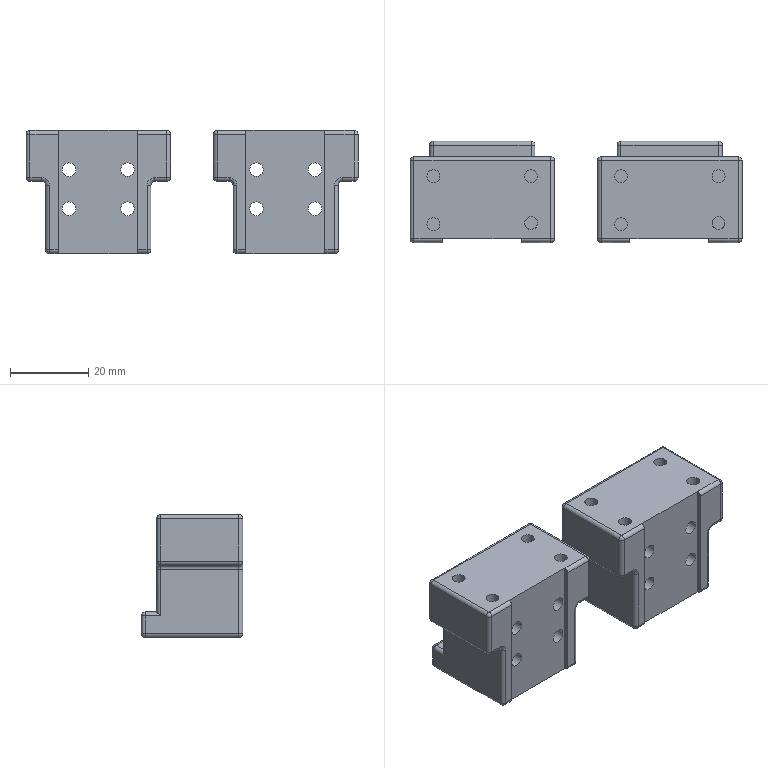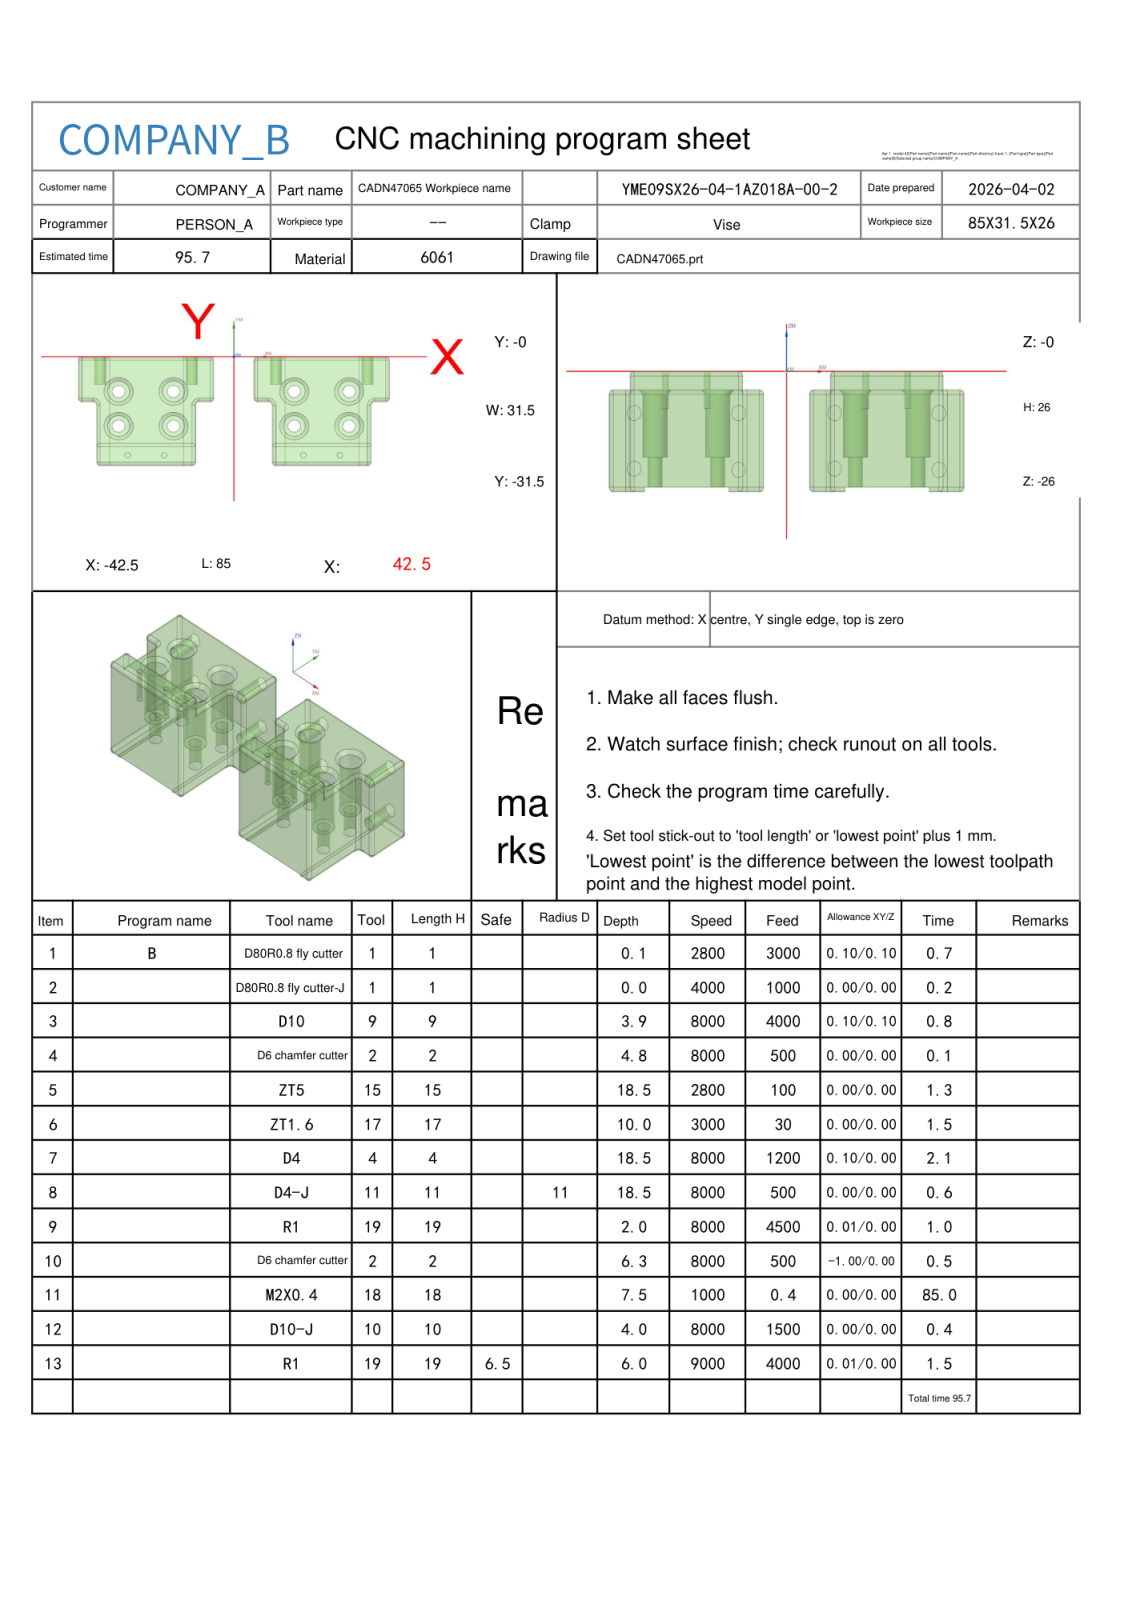NC program | NX | posted by the shop | part box 85 x 26 x 31.5 mm
Lines 10969 to 12542 of 12542:
N10 T02 M06
(D6 chamfer cutter  D=6. R=0. H=02 ce=0.00 di=0.00)
G00 G90 G54 X-29.011 Y-28.455 M03 S8000
G43 H02 Z20.
M08
G98 G81 X-29.011 Y-28.455 Z-1.2 R3. F500.
X-19.011
X18.989
X28.989
G80
G00 Z20.
G00 G90 X-33.191 Y-20.222 M03 S8000
Z20.
Z-1.5
G01 X-33.173 Y-20.379 Z-1.558 F500.
X-33.097 Y-20.648 Z-1.659
X-32.977 Y-20.902 Z-1.761
X-32.818 Y-21.132 Z-1.863
X-32.623 Y-21.333 Z-1.965
X-32.397 Y-21.499 Z-2.067
X-32.148 Y-21.626 Z-2.169
X-31.881 Y-21.71 Z-2.271
X-31.604 Y-21.75 Z-2.373
X-31.401 Z-2.447
X-31.124 Y-21.71 Z-2.548
X-30.857 Y-21.626 Z-2.65
X-30.608 Y-21.499 Z-2.752
X-30.382 Y-21.333 Z-2.854
X-30.187 Y-21.132 Z-2.956
X-30.028 Y-20.902 Z-3.058
X-29.908 Y-20.648 Z-3.16
X-29.832 Y-20.379 Z-3.262
X-29.8 Y-20.101 Z-3.364
X-29.815 Y-19.821 Z-3.466
X-29.875 Y-19.547 Z-3.568
X-29.98 Y-19.288 Z-3.67
X-30.081 Y-19.113 Z-3.743
X-30.254 Y-18.892 Z-3.845
X-30.46 Y-18.703 Z-3.947
X-30.695 Y-18.551 Z-4.049
X-30.952 Y-18.439 Z-4.151
X-31.223 Y-18.37 Z-4.253
X-31.502 Y-18.347 Z-4.355
X-31.782 Y-18.37 Z-4.457
X-32.053 Y-18.439 Z-4.559
X-32.31 Y-18.551 Z-4.661
X-32.545 Y-18.703 Z-4.763
X-32.751 Y-18.892 Z-4.865
X-32.924 Y-19.113 Z-4.967
X-33.025 Y-19.288 Z-5.04
X-33.13 Y-19.547 Z-5.142
X-33.19 Y-19.821 Z-5.244
X-33.205 Y-20.101 Z-5.346
X-33.173 Y-20.379 Z-5.448
X-33.097 Y-20.648 Z-5.55
X-32.977 Y-20.902 Z-5.652
X-32.818 Y-21.132 Z-5.754
X-32.623 Y-21.333 Z-5.856
X-32.397 Y-21.499 Z-5.957
X-32.148 Y-21.626 Z-6.059
X-31.881 Y-21.71 Z-6.161
X-31.604 Y-21.75 Z-6.263
X-31.502 Z-6.3
G03 X-29.802 Y-20.05 I0.0 J1.7
X-31.502 Y-18.35 I-1.7 J0.0
X-33.202 Y-20.05 I0.0 J-1.7
X-31.502 Y-21.75 I1.7 J0.0
X-31.01 Y-21.677 I0.0 J1.7
G01 Z-3.8
G00 Z20.
X-33.191 Y-10.222
Z-1.5
G01 X-33.173 Y-10.379 Z-1.558
X-33.097 Y-10.648 Z-1.659
X-32.977 Y-10.902 Z-1.761
X-32.818 Y-11.132 Z-1.863
X-32.623 Y-11.333 Z-1.965
X-32.397 Y-11.499 Z-2.067
X-32.148 Y-11.626 Z-2.169
X-31.881 Y-11.71 Z-2.271
X-31.604 Y-11.75 Z-2.373
X-31.401 Z-2.447
X-31.124 Y-11.71 Z-2.548
X-30.857 Y-11.626 Z-2.65
X-30.608 Y-11.499 Z-2.752
X-30.382 Y-11.333 Z-2.854
X-30.187 Y-11.132 Z-2.956
X-30.028 Y-10.902 Z-3.058
X-29.908 Y-10.648 Z-3.16
X-29.832 Y-10.379 Z-3.262
X-29.8 Y-10.101 Z-3.364
X-29.815 Y-9.821 Z-3.466
X-29.875 Y-9.547 Z-3.568
X-29.98 Y-9.288 Z-3.67
X-30.081 Y-9.113 Z-3.743
X-30.254 Y-8.892 Z-3.845
X-30.46 Y-8.703 Z-3.947
X-30.695 Y-8.551 Z-4.049
X-30.952 Y-8.439 Z-4.151
X-31.223 Y-8.37 Z-4.253
X-31.502 Y-8.347 Z-4.355
X-31.782 Y-8.37 Z-4.457
X-32.053 Y-8.439 Z-4.559
X-32.31 Y-8.551 Z-4.661
X-32.545 Y-8.703 Z-4.763
X-32.751 Y-8.892 Z-4.865
X-32.924 Y-9.113 Z-4.967
X-33.025 Y-9.288 Z-5.04
X-33.13 Y-9.547 Z-5.142
X-33.19 Y-9.821 Z-5.244
X-33.205 Y-10.101 Z-5.346
X-33.173 Y-10.379 Z-5.448
X-33.097 Y-10.648 Z-5.55
X-32.977 Y-10.902 Z-5.652
X-32.818 Y-11.132 Z-5.754
X-32.623 Y-11.333 Z-5.856
X-32.397 Y-11.499 Z-5.957
X-32.148 Y-11.626 Z-6.059
X-31.881 Y-11.71 Z-6.161
X-31.604 Y-11.75 Z-6.263
X-31.502 Z-6.3
G03 X-29.802 Y-10.05 I0.0 J1.7
X-31.502 Y-8.35 I-1.7 J0.0
X-33.202 Y-10.05 I0.0 J-1.7
X-31.502 Y-11.75 I1.7 J0.0
X-31.01 Y-11.677 I0.0 J1.7
G01 Z-3.8
G00 Z20.
X-18.191 Y-10.222
Z-1.5
G01 X-18.173 Y-10.379 Z-1.558
X-18.097 Y-10.648 Z-1.659
X-17.977 Y-10.902 Z-1.761
X-17.818 Y-11.132 Z-1.863
X-17.623 Y-11.333 Z-1.965
X-17.397 Y-11.499 Z-2.067
X-17.148 Y-11.626 Z-2.169
X-16.881 Y-11.71 Z-2.271
X-16.604 Y-11.75 Z-2.373
X-16.401 Z-2.447
X-16.124 Y-11.71 Z-2.548
X-15.857 Y-11.626 Z-2.65
X-15.608 Y-11.499 Z-2.752
X-15.382 Y-11.333 Z-2.854
X-15.187 Y-11.132 Z-2.956
X-15.028 Y-10.902 Z-3.058
X-14.908 Y-10.648 Z-3.16
X-14.832 Y-10.379 Z-3.262
X-14.8 Y-10.101 Z-3.364
X-14.815 Y-9.821 Z-3.466
X-14.875 Y-9.547 Z-3.568
X-14.98 Y-9.288 Z-3.67
X-15.081 Y-9.113 Z-3.743
X-15.254 Y-8.892 Z-3.845
X-15.46 Y-8.703 Z-3.947
X-15.695 Y-8.551 Z-4.049
X-15.952 Y-8.439 Z-4.151
X-16.223 Y-8.37 Z-4.253
X-16.502 Y-8.347 Z-4.355
X-16.782 Y-8.37 Z-4.457
X-17.053 Y-8.439 Z-4.559
X-17.31 Y-8.551 Z-4.661
X-17.545 Y-8.703 Z-4.763
X-17.751 Y-8.892 Z-4.865
X-17.924 Y-9.113 Z-4.967
X-18.025 Y-9.288 Z-5.04
X-18.13 Y-9.547 Z-5.142
X-18.19 Y-9.821 Z-5.244
X-18.205 Y-10.101 Z-5.346
X-18.173 Y-10.379 Z-5.448
X-18.097 Y-10.648 Z-5.55
X-17.977 Y-10.902 Z-5.652
X-17.818 Y-11.132 Z-5.754
X-17.623 Y-11.333 Z-5.856
X-17.397 Y-11.499 Z-5.957
X-17.148 Y-11.626 Z-6.059
X-16.881 Y-11.71 Z-6.161
X-16.604 Y-11.75 Z-6.263
X-16.502 Z-6.3
G03 X-14.802 Y-10.05 I0.0 J1.7
X-16.502 Y-8.35 I-1.7 J0.0
X-18.202 Y-10.05 I0.0 J-1.7
X-16.502 Y-11.75 I1.7 J0.0
X-16.01 Y-11.677 I0.0 J1.7
G01 Z-3.8
G00 Z20.
X-18.191 Y-20.222
Z-1.5
G01 X-18.173 Y-20.379 Z-1.558
X-18.097 Y-20.648 Z-1.659
X-17.977 Y-20.902 Z-1.761
X-17.818 Y-21.132 Z-1.863
X-17.623 Y-21.333 Z-1.965
X-17.397 Y-21.499 Z-2.067
X-17.148 Y-21.626 Z-2.169
X-16.881 Y-21.71 Z-2.271
X-16.604 Y-21.75 Z-2.373
X-16.401 Z-2.447
X-16.124 Y-21.71 Z-2.548
X-15.857 Y-21.626 Z-2.65
X-15.608 Y-21.499 Z-2.752
X-15.382 Y-21.333 Z-2.854
X-15.187 Y-21.132 Z-2.956
X-15.028 Y-20.902 Z-3.058
X-14.908 Y-20.648 Z-3.16
X-14.832 Y-20.379 Z-3.262
X-14.8 Y-20.101 Z-3.364
X-14.815 Y-19.821 Z-3.466
X-14.875 Y-19.547 Z-3.568
X-14.98 Y-19.288 Z-3.67
X-15.081 Y-19.113 Z-3.743
X-15.254 Y-18.892 Z-3.845
X-15.46 Y-18.703 Z-3.947
X-15.695 Y-18.551 Z-4.049
X-15.952 Y-18.439 Z-4.151
X-16.223 Y-18.37 Z-4.253
X-16.502 Y-18.347 Z-4.355
X-16.782 Y-18.37 Z-4.457
X-17.053 Y-18.439 Z-4.559
X-17.31 Y-18.551 Z-4.661
X-17.545 Y-18.703 Z-4.763
X-17.751 Y-18.892 Z-4.865
X-17.924 Y-19.113 Z-4.967
X-18.025 Y-19.288 Z-5.04
X-18.13 Y-19.547 Z-5.142
X-18.19 Y-19.821 Z-5.244
X-18.205 Y-20.101 Z-5.346
X-18.173 Y-20.379 Z-5.448
X-18.097 Y-20.648 Z-5.55
X-17.977 Y-20.902 Z-5.652
X-17.818 Y-21.132 Z-5.754
X-17.623 Y-21.333 Z-5.856
X-17.397 Y-21.499 Z-5.957
X-17.148 Y-21.626 Z-6.059
X-16.881 Y-21.71 Z-6.161
X-16.604 Y-21.75 Z-6.263
X-16.502 Z-6.3
G03 X-14.802 Y-20.05 I0.0 J1.7
X-16.502 Y-18.35 I-1.7 J0.0
X-18.202 Y-20.05 I0.0 J-1.7
X-16.502 Y-21.75 I1.7 J0.0
X-16.01 Y-21.677 I0.0 J1.7
G01 Z-3.8
G00 Z20.
X14.809 Y-20.222
Z-1.5
G01 X14.827 Y-20.379 Z-1.558
X14.903 Y-20.648 Z-1.659
X15.023 Y-20.902 Z-1.761
X15.182 Y-21.132 Z-1.863
X15.377 Y-21.333 Z-1.965
X15.603 Y-21.499 Z-2.067
X15.852 Y-21.626 Z-2.169
X16.119 Y-21.71 Z-2.271
X16.396 Y-21.75 Z-2.373
X16.599 Z-2.447
X16.876 Y-21.71 Z-2.548
X17.143 Y-21.626 Z-2.65
X17.392 Y-21.499 Z-2.752
X17.618 Y-21.333 Z-2.854
X17.813 Y-21.132 Z-2.956
X17.972 Y-20.902 Z-3.058
X18.092 Y-20.648 Z-3.16
X18.168 Y-20.379 Z-3.262
X18.2 Y-20.101 Z-3.364
X18.185 Y-19.821 Z-3.466
X18.125 Y-19.547 Z-3.568
X18.02 Y-19.288 Z-3.67
X17.919 Y-19.113 Z-3.743
X17.746 Y-18.892 Z-3.845
X17.54 Y-18.703 Z-3.947
X17.305 Y-18.551 Z-4.049
X17.048 Y-18.439 Z-4.151
X16.777 Y-18.37 Z-4.253
X16.498 Y-18.347 Z-4.355
X16.218 Y-18.37 Z-4.457
X15.947 Y-18.439 Z-4.559
X15.69 Y-18.551 Z-4.661
X15.455 Y-18.703 Z-4.763
X15.249 Y-18.892 Z-4.865
X15.076 Y-19.113 Z-4.967
X14.975 Y-19.288 Z-5.04
X14.87 Y-19.547 Z-5.142
X14.81 Y-19.821 Z-5.244
X14.795 Y-20.101 Z-5.346
X14.827 Y-20.379 Z-5.448
X14.903 Y-20.648 Z-5.55
X15.023 Y-20.902 Z-5.652
X15.182 Y-21.132 Z-5.754
X15.377 Y-21.333 Z-5.856
X15.603 Y-21.499 Z-5.957
X15.852 Y-21.626 Z-6.059
X16.119 Y-21.71 Z-6.161
X16.396 Y-21.75 Z-6.263
X16.498 Z-6.3
G03 X18.198 Y-20.05 I0.0 J1.7
X16.498 Y-18.35 I-1.7 J0.0
X14.798 Y-20.05 I0.0 J-1.7
X16.498 Y-21.75 I1.7 J0.0
X16.99 Y-21.677 I0.0 J1.7
G01 Z-3.8
G00 Z20.
X14.809 Y-10.222
Z-1.5
G01 X14.827 Y-10.379 Z-1.558
X14.903 Y-10.648 Z-1.659
X15.023 Y-10.902 Z-1.761
X15.182 Y-11.132 Z-1.863
X15.377 Y-11.333 Z-1.965
X15.603 Y-11.499 Z-2.067
X15.852 Y-11.626 Z-2.169
X16.119 Y-11.71 Z-2.271
X16.396 Y-11.75 Z-2.373
X16.599 Z-2.447
X16.876 Y-11.71 Z-2.548
X17.143 Y-11.626 Z-2.65
X17.392 Y-11.499 Z-2.752
X17.618 Y-11.333 Z-2.854
X17.813 Y-11.132 Z-2.956
X17.972 Y-10.902 Z-3.058
X18.092 Y-10.648 Z-3.16
X18.168 Y-10.379 Z-3.262
X18.2 Y-10.101 Z-3.364
X18.185 Y-9.821 Z-3.466
X18.125 Y-9.547 Z-3.568
X18.02 Y-9.288 Z-3.67
X17.919 Y-9.113 Z-3.743
X17.746 Y-8.892 Z-3.845
X17.54 Y-8.703 Z-3.947
X17.305 Y-8.551 Z-4.049
X17.048 Y-8.439 Z-4.151
X16.777 Y-8.37 Z-4.253
X16.498 Y-8.347 Z-4.355
X16.218 Y-8.37 Z-4.457
X15.947 Y-8.439 Z-4.559
X15.69 Y-8.551 Z-4.661
X15.455 Y-8.703 Z-4.763
X15.249 Y-8.892 Z-4.865
X15.076 Y-9.113 Z-4.967
X14.975 Y-9.288 Z-5.04
X14.87 Y-9.547 Z-5.142
X14.81 Y-9.821 Z-5.244
X14.795 Y-10.101 Z-5.346
X14.827 Y-10.379 Z-5.448
X14.903 Y-10.648 Z-5.55
X15.023 Y-10.902 Z-5.652
X15.182 Y-11.132 Z-5.754
X15.377 Y-11.333 Z-5.856
X15.603 Y-11.499 Z-5.957
X15.852 Y-11.626 Z-6.059
X16.119 Y-11.71 Z-6.161
X16.396 Y-11.75 Z-6.263
X16.498 Z-6.3
G03 X18.198 Y-10.05 I0.0 J1.7
X16.498 Y-8.35 I-1.7 J0.0
X14.798 Y-10.05 I0.0 J-1.7
X16.498 Y-11.75 I1.7 J0.0
X16.99 Y-11.677 I0.0 J1.7
G01 Z-3.8
G00 Z20.
X29.809 Y-10.222
Z-1.5
G01 X29.827 Y-10.379 Z-1.558
X29.903 Y-10.648 Z-1.659
X30.023 Y-10.902 Z-1.761
X30.182 Y-11.132 Z-1.863
X30.377 Y-11.333 Z-1.965
X30.603 Y-11.499 Z-2.067
X30.852 Y-11.626 Z-2.169
X31.119 Y-11.71 Z-2.271
X31.396 Y-11.75 Z-2.373
X31.599 Z-2.447
X31.876 Y-11.71 Z-2.548
X32.143 Y-11.626 Z-2.65
X32.392 Y-11.499 Z-2.752
X32.618 Y-11.333 Z-2.854
X32.813 Y-11.132 Z-2.956
X32.972 Y-10.902 Z-3.058
X33.092 Y-10.648 Z-3.16
X33.168 Y-10.379 Z-3.262
X33.2 Y-10.101 Z-3.364
X33.185 Y-9.821 Z-3.466
X33.125 Y-9.547 Z-3.568
X33.02 Y-9.288 Z-3.67
X32.919 Y-9.113 Z-3.743
X32.746 Y-8.892 Z-3.845
X32.54 Y-8.703 Z-3.947
X32.305 Y-8.551 Z-4.049
X32.048 Y-8.439 Z-4.151
X31.777 Y-8.37 Z-4.253
X31.498 Y-8.347 Z-4.355
X31.218 Y-8.37 Z-4.457
X30.947 Y-8.439 Z-4.559
X30.69 Y-8.551 Z-4.661
X30.455 Y-8.703 Z-4.763
X30.249 Y-8.892 Z-4.865
X30.076 Y-9.113 Z-4.967
X29.975 Y-9.288 Z-5.04
X29.87 Y-9.547 Z-5.142
X29.81 Y-9.821 Z-5.244
X29.795 Y-10.101 Z-5.346
X29.827 Y-10.379 Z-5.448
X29.903 Y-10.648 Z-5.55
X30.023 Y-10.902 Z-5.652
X30.182 Y-11.132 Z-5.754
X30.377 Y-11.333 Z-5.856
X30.603 Y-11.499 Z-5.957
X30.852 Y-11.626 Z-6.059
X31.119 Y-11.71 Z-6.161
X31.396 Y-11.75 Z-6.263
X31.498 Z-6.3
G03 X33.198 Y-10.05 I0.0 J1.7
X31.498 Y-8.35 I-1.7 J0.0
X29.798 Y-10.05 I0.0 J-1.7
X31.498 Y-11.75 I1.7 J0.0
X31.99 Y-11.677 I0.0 J1.7
G01 Z-3.8
G00 Z20.
X29.809 Y-20.222
Z-1.5
G01 X29.827 Y-20.379 Z-1.558
X29.903 Y-20.648 Z-1.659
X30.023 Y-20.902 Z-1.761
X30.182 Y-21.132 Z-1.863
X30.377 Y-21.333 Z-1.965
X30.603 Y-21.499 Z-2.067
X30.852 Y-21.626 Z-2.169
X31.119 Y-21.71 Z-2.271
X31.396 Y-21.75 Z-2.373
X31.599 Z-2.447
X31.876 Y-21.71 Z-2.548
X32.143 Y-21.626 Z-2.65
X32.392 Y-21.499 Z-2.752
X32.618 Y-21.333 Z-2.854
X32.813 Y-21.132 Z-2.956
X32.972 Y-20.902 Z-3.058
X33.092 Y-20.648 Z-3.16
X33.168 Y-20.379 Z-3.262
X33.2 Y-20.101 Z-3.364
X33.185 Y-19.821 Z-3.466
X33.125 Y-19.547 Z-3.568
X33.02 Y-19.288 Z-3.67
X32.919 Y-19.113 Z-3.743
X32.746 Y-18.892 Z-3.845
X32.54 Y-18.703 Z-3.947
X32.305 Y-18.551 Z-4.049
X32.048 Y-18.439 Z-4.151
X31.777 Y-18.37 Z-4.253
X31.498 Y-18.347 Z-4.355
X31.218 Y-18.37 Z-4.457
X30.947 Y-18.439 Z-4.559
X30.69 Y-18.551 Z-4.661
X30.455 Y-18.703 Z-4.763
X30.249 Y-18.892 Z-4.865
X30.076 Y-19.113 Z-4.967
X29.975 Y-19.288 Z-5.04
X29.87 Y-19.547 Z-5.142
X29.81 Y-19.821 Z-5.244
X29.795 Y-20.101 Z-5.346
X29.827 Y-20.379 Z-5.448
X29.903 Y-20.648 Z-5.55
X30.023 Y-20.902 Z-5.652
X30.182 Y-21.132 Z-5.754
X30.377 Y-21.333 Z-5.856
X30.603 Y-21.499 Z-5.957
X30.852 Y-21.626 Z-6.059
X31.119 Y-21.71 Z-6.161
X31.396 Y-21.75 Z-6.263
X31.498 Z-6.3
G03 X33.198 Y-20.05 I0.0 J1.7
X31.498 Y-18.35 I-1.7 J0.0
X29.798 Y-20.05 I0.0 J-1.7
X31.498 Y-21.75 I1.7 J0.0
X31.99 Y-21.677 I0.0 J1.7
G01 Z-3.8
G00 Z20.
G91 G28 Z0.0
M05
M09
G91 G28 Z0.0
M01
N11 T18 M06
(M2X0.4 D=1.6 DR_a=180 H=18)
G00 G90 G54 X-29.011 Y-28.455 M03 S1000
G43 H18 Z20.
M08
G95
G98 G84 X-29.011 Y-28.455 Z-7.5 R1. F.4 Q2.
X-19.011
X18.989
X28.989
G80
G94
G00 Z20.
G91 G28 Z0.0
M05
M09
G91 G28 Z0.0
M01
N12 T10 M06
(D10-J  D=10. R=0. H=10 ce=0.40 di=0.00)
G00 G90 G54 X-48.5 Y1.999 M03 S7000
G43 H10 Z13.8
M08
Z-2.5
G01 Z-4. F1500.
G03 X-46.5 Y0.0 I2. J0.0
G01 X45.6
G02 X46.5 Y-.9 I0.0 J-.9
G01 Y-3.889
G02 X45.5 Y-4.889 I-1. J0.0
G01 X-45.6
G03 X-46.5 Y-5.789 I0.0 J-.9
G01 Y-8.778
G03 X-45.5 Y-9.778 I1. J0.0
G01 X45.6
G02 X46.5 Y-10.678 I0.0 J-.9
G01 Y-13.666
G02 X45.5 Y-14.666 I-1. J0.0
G01 X-45.501
G03 X-46.5 Y-15.666 I.001 J-1.
G01 Y-16.388
G03 X-45.955 Y-17.278 I1. J0.0
G01 X-41.714 Y-19.446
G03 X-41.26 Y-19.555 I.455 J.891
G01 X41.5
G03 X42.5 Y-18.555 I0.0 J1.
G01 X43.5 Y-19.
Z-2.5
G00 Z13.8
G00 G90 X3.8 Y-27.455 M03 S8000
Z8.8
Z-3.
G01 Z-4. F1000.
G41 D10
X4.
G03 X5.5 Y-25.955 I0.0 J1.5
G02 X11.5 Y-19.955 I6. J0.0
G01 X36.5
G02 X42.5 Y-25.955 I0.0 J-6.
G03 X44. Y-27.455 I1.5 J0.0
G01 G40 X44.2
Z-3.
G00 Z8.8
X-44.2
Z-3.
G01 Z-4.
G41 D10
X-44.
G03 X-42.5 Y-25.955 I0.0 J1.5
G02 X-36.5 Y-19.955 I6. J0.0
G01 X-11.5
G02 X-5.5 Y-25.955 I0.0 J-6.
G03 X-4. Y-27.455 I1.5 J0.0
G01 G40 X-3.8
Z-3.
G00 Z8.8
G91 G28 Z0.0
M05
M09
G91 G28 Z0.0
M01
N13 T19 M06
(R1  D=2. R=1. H=19 ce=0.01 di=0.00)
G00 G90 G54 X10.223 Y-23.23 M03 S9000
G43 H19 Z13.8
M08
Z-3.51
G01 Z-4.01 F4000.
G03 X11.186 Y-23.962 I.963 J.268
G01 X11.291 Y-23.956
Y-14.
G03 X9.5 Y-12.209 I-1.791 J0.0
G01 X6.5
G02 X6.291 Y-12. I0.0 J.209
G01 Y-1.
G02 X6.5 Y-.791 I.209 J0.0
G01 X41.5
G02 X41.709 Y-1. I0.0 J-.209
G01 Y-12.
G02 X41.5 Y-12.209 I-.209 J0.0
G01 X38.5
G03 X36.709 Y-14. I0.0 J-1.791
G01 Y-23.956
X36.774 Y-23.964 Z-4.018
X36.825 Y-23.972 Z-4.025
Y-14.
G02 X38.5 Y-12.325 I1.675 J0.0
G01 X41.5
G03 X41.825 Y-12. I0.0 J.325
G01 Y-1.
G03 X41.5 Y-.675 I-.325 J0.0
G01 X6.5
G03 X6.175 Y-1. I0.0 J-.325
G01 Y-12.
G03 X6.5 Y-12.325 I.325 J0.0
G01 X9.5
G02 X11.175 Y-14. I0.0 J-1.675
G01 Y-23.972
X11.119 Y-23.982 Z-4.035
X11.07 Y-23.992 Z-4.045
Y-14.
G03 X9.5 Y-12.43 I-1.57 J0.0
G01 X6.5
G02 X6.07 Y-12. I0.0 J.43
G01 Y-1.
G02 X6.5 Y-.57 I.43 J0.0
G01 X41.5
G02 X41.93 Y-1. I0.0 J-.43
G01 Y-12.
G02 X41.5 Y-12.43 I-.43 J0.0
G01 X38.5
G03 X36.93 Y-14. I0.0 J-1.57
G01 Y-23.992
X37.01 Y-24.011 Z-4.069
Y-14.
G02 X38.5 Y-12.51 I1.49 J0.0
G01 X41.5
G03 X42.01 Y-12. I0.0 J.51
G01 Y-1.
G03 X41.5 Y-.49 I-.51 J0.0
G01 X6.5
G03 X5.99 Y-1. I0.0 J-.51
G01 Y-12.
G03 X6.5 Y-12.51 I.51 J0.0
G01 X9.5
G02 X10.99 Y-14. I0.0 J-1.49
G01 Y-24.011
X10.918 Y-24.027 Z-4.084
X10.879 Y-24.044 Z-4.098
Y-14.
G03 X9.5 Y-12.621 I-1.379 J0.0
G01 X6.5
G02 X5.879 Y-12. I0.0 J.621
G01 Y-1.
G02 X6.5 Y-.379 I.621 J0.0
G01 X41.5
G02 X42.121 Y-1. I0.0 J-.621
G01 Y-12.
G02 X41.5 Y-12.621 I-.621 J0.0
G01 X38.5
G03 X37.121 Y-14. I0.0 J-1.379
G01 Y-24.044
X37.18 Y-24.062 Z-4.115
X37.226 Y-24.081 Z-4.133
Y-14.
G02 X38.5 Y-12.726 I1.274 J0.0
G01 X41.5
G03 X42.226 Y-12. I0.0 J.726
G01 Y-1.
G03 X41.5 Y-.274 I-.726 J0.0
G01 X6.5
G03 X5.774 Y-1. I0.0 J-.726
G01 Y-12.
G03 X6.5 Y-12.726 I.726 J0.0
G01 X9.5
G02 X10.774 Y-14. I0.0 J-1.274
G01 Y-24.081
X10.726 Y-24.1 Z-4.152
X10.68 Y-24.12 Z-4.171
Y-14.
G03 X9.5 Y-12.82 I-1.18 J0.0
G01 X6.5
G02 X5.68 Y-12. I0.0 J.82
G01 Y-1.
G02 X6.5 Y-.18 I.82 J0.0
G01 X41.5
G02 X42.32 Y-1. I0.0 J-.82
G01 Y-12.
G02 X41.5 Y-12.82 I-.82 J0.0
G01 X38.5
G03 X37.32 Y-14. I0.0 J-1.18
G01 Y-24.12
X37.367 Y-24.142 Z-4.193
X37.411 Y-24.164 Z-4.215
Y-14.
G02 X38.5 Y-12.911 I1.089 J0.0
G01 X41.5
G03 X42.411 Y-12. I0.0 J.911
G01 Y-1.
G03 X41.5 Y-.089 I-.911 J0.0
G01 X6.5
G03 X5.589 Y-1. I0.0 J-.911
G01 Y-12.
G03 X6.5 Y-12.911 I.911 J0.0
G01 X9.5
G02 X10.589 Y-14. I0.0 J-1.089
G01 Y-24.164
X10.543 Y-24.188 Z-4.238
X10.5 Y-24.212 Z-4.262
Y-14.
G03 X9.5 Y-13. I-1. J0.0
G01 X6.5
G02 X5.5 Y-12. I0.0 J1.
G01 Y-1.
G02 X6.5 Y0.0 I1. J0.0
G01 X41.5
G02 X42.5 Y-1. I0.0 J-1.
G01 Y-12.
G02 X41.5 Y-13. I-1. J0.0
G01 X38.5
G03 X37.5 Y-14. I0.0 J-1.
G01 Y-24.212
X37.544 Y-24.238 Z-4.288
X37.586 Y-24.264 Z-4.314
Y-14.
G02 X38.5 Y-13.086 I.914 J0.0
G01 X41.5
G03 X42.586 Y-12. I0.0 J1.086
G01 Y-1.
G03 X41.5 Y.086 I-1.086 J0.0
G01 X6.5
G03 X5.414 Y-1. I0.0 J-1.086
G01 Y-12.
G03 X6.5 Y-13.086 I1.086 J0.0
G01 X9.5
G02 X10.414 Y-14. I0.0 J-.914
G01 Y-24.264
X10.371 Y-24.292 Z-4.343
X10.33 Y-24.321 Z-4.371
Y-14.
G03 X9.5 Y-13.17 I-.83 J0.0
G01 X6.5
G02 X5.33 Y-12. I0.0 J1.17
G01 Y-1.
G02 X6.5 Y.17 I1.17 J0.0
G01 X41.5
G02 X42.67 Y-1. I0.0 J-1.17
G01 Y-12.
G02 X41.5 Y-13.17 I-1.17 J0.0
G01 X38.5
G03 X37.67 Y-14. I0.0 J-.83
G01 Y-24.321
X37.711 Y-24.351 Z-4.401
X37.75 Y-24.381 Z-4.431
Y-14.
G02 X38.5 Y-13.25 I.75 J0.0
G01 X41.5
G03 X42.75 Y-12. I0.0 J1.25
G01 Y-1.
G03 X41.5 Y.25 I-1.25 J0.0
G01 X6.5
G03 X5.25 Y-1. I0.0 J-1.25
G01 Y-12.
G03 X6.5 Y-13.25 I1.25 J0.0
G01 X9.5
G02 X10.25 Y-14. I0.0 J-.75
G01 Y-24.381
X10.21 Y-24.414 Z-4.463
X10.173 Y-24.446 Z-4.495
Y-14.
G03 X9.5 Y-13.327 I-.673 J0.0
G01 X6.5
G02 X5.173 Y-12. I0.0 J1.327
G01 Y-1.
G02 X6.5 Y.327 I1.327 J0.0
G01 X41.5
G02 X42.827 Y-1. I0.0 J-1.327
G01 Y-12.
G02 X41.5 Y-13.327 I-1.327 J0.0
G01 X38.5
G03 X37.827 Y-14. I0.0 J-.673
G01 Y-24.446
X37.865 Y-24.48 Z-4.529
X37.901 Y-24.514 Z-4.563
Y-14.
G02 X38.5 Y-13.401 I.599 J0.0
G01 X41.5
G03 X42.901 Y-12. I0.0 J1.401
G01 Y-1.
G03 X41.5 Y.401 I-1.401 J0.0
G01 X6.5
G03 X5.099 Y-1. I0.0 J-1.401
G01 Y-12.
G03 X6.5 Y-13.401 I1.401 J0.0
G01 X9.5
G02 X10.099 Y-14. I0.0 J-.599
G01 Y-24.514
X10.063 Y-24.55 Z-4.599
X10.028 Y-24.586 Z-4.635
Y-14.
G03 X9.5 Y-13.472 I-.528 J0.0
G01 X6.5
G02 X5.028 Y-12. I0.0 J1.472
G01 Y-1.
G02 X6.5 Y.472 I1.472 J0.0
G01 X41.5
G02 X42.972 Y-1. I0.0 J-1.472
G01 Y-12.
G02 X41.5 Y-13.472 I-1.472 J0.0
G01 X38.5
G03 X37.972 Y-14. I0.0 J-.528
G01 Y-24.586
X38.006 Y-24.624 Z-4.672
X38.038 Y-24.661 Z-4.71
Y-14.
G02 X38.5 Y-13.538 I.462 J0.0
G01 X41.5
G03 X43.038 Y-12. I0.0 J1.538
G01 Y-1.
G03 X41.5 Y.538 I-1.538 J0.0
G01 X6.5
G03 X4.962 Y-1. I0.0 J-1.538
G01 Y-12.
G03 X6.5 Y-13.538 I1.538 J0.0
G01 X9.5
G02 X9.962 Y-14. I0.0 J-.462
G01 Y-24.661
X9.899 Y-24.74 Z-4.788
Y-14.
G03 X9.5 Y-13.601 I-.399 J0.0
G01 X6.5
G02 X4.899 Y-12. I0.0 J1.601
G01 Y-1.
G02 X6.5 Y.601 I1.601 J0.0
G01 X41.5
G02 X43.101 Y-1. I0.0 J-1.601
G01 Y-12.
G02 X41.5 Y-13.601 I-1.601 J0.0
G01 X38.5
G03 X38.101 Y-14. I0.0 J-.399
G01 Y-24.74
X38.16 Y-24.821 Z-4.869
Y-14.
G02 X38.5 Y-13.66 I.34 J0.0
G01 X41.5
G03 X43.16 Y-12. I0.0 J1.66
G01 Y-1.
G03 X41.5 Y.66 I-1.66 J0.0
G01 X6.5
G03 X4.84 Y-1. I0.0 J-1.66
G01 Y-12.
G03 X6.5 Y-13.66 I1.66 J0.0
G01 X9.5
G02 X9.84 Y-14. I0.0 J-.34
G01 Y-24.821
X9.786 Y-24.906 Z-4.953
Y-14.
G03 X9.5 Y-13.714 I-.286 J0.0
G01 X6.5
G02 X4.786 Y-12. I0.0 J1.714
G01 Y-1.
G02 X6.5 Y.714 I1.714 J0.0
G01 X41.5
G02 X43.214 Y-1. I0.0 J-1.714
G01 Y-12.
G02 X41.5 Y-13.714 I-1.714 J0.0
G01 X38.5
G03 X38.214 Y-14. I0.0 J-.286
G01 Y-24.906
X38.264 Y-24.993 Z-5.04
Y-14.
G02 X38.5 Y-13.764 I.236 J0.0
G01 X41.5
G03 X43.264 Y-12. I0.0 J1.764
G01 Y-1.
G03 X41.5 Y.764 I-1.764 J0.0
G01 X6.5
G03 X4.736 Y-1. I0.0 J-1.764
G01 Y-12.
G03 X6.5 Y-13.764 I1.764 J0.0
G01 X9.5
G02 X9.736 Y-14. I0.0 J-.236
G01 Y-24.993
X9.69 Y-25.082 Z-5.129
Y-14.
G03 X9.5 Y-13.81 I-.19 J0.0
G01 X6.5
G02 X4.69 Y-12. I0.0 J1.81
G01 Y-1.
G02 X6.5 Y.81 I1.81 J0.0
G01 X41.5
G02 X43.31 Y-1. I0.0 J-1.81
G01 Y-12.
G02 X41.5 Y-13.81 I-1.81 J0.0
G01 X38.5
G03 X38.31 Y-14. I0.0 J-.19
G01 Y-25.082
X38.352 Y-25.173 Z-5.22
Y-14.
G02 X38.5 Y-13.852 I.148 J0.0
G01 X41.5
G03 X43.352 Y-12. I0.0 J1.852
G01 Y-1.
G03 X41.5 Y.852 I-1.852 J0.0
G01 X6.5
G03 X4.648 Y-1. I0.0 J-1.852
G01 Y-12.
G03 X6.5 Y-13.852 I1.852 J0.0
G01 X9.5
G02 X9.648 Y-14. I0.0 J-.148
G01 Y-25.173
X9.612 Y-25.267 Z-5.313
Y-14.
X9.605 Y-13.939
X9.561 Y-13.895
X9.5 Y-13.888
X6.5
G02 X4.612 Y-12. I0.0 J1.888
G01 Y-1.
G02 X6.5 Y.888 I1.888 J0.0
G01 X41.5
G02 X43.388 Y-1. I0.0 J-1.888
G01 Y-12.
G02 X41.5 Y-13.888 I-1.888 J0.0
G01 X38.5
X38.439 Y-13.895
X38.395 Y-13.939
X38.388 Y-14.
Y-25.267
X38.42 Y-25.362 Z-5.408
Y-14.
X38.422 Y-13.955
X38.455 Y-13.922
X38.5 Y-13.92
X41.5
G03 X43.42 Y-12. I0.0 J1.92
G01 Y-1.
G03 X41.5 Y.92 I-1.92 J0.0
G01 X6.5
G03 X4.58 Y-1. I0.0 J-1.92
G01 Y-12.
G03 X6.5 Y-13.92 I1.92 J0.0
G01 X9.5
X9.545 Y-13.922
X9.578 Y-13.955
X9.58 Y-14.
Y-25.362
X9.552 Y-25.458 Z-5.504
Y-14.
X9.554 Y-13.969
X9.531 Y-13.946
X9.5 Y-13.948
X6.5
G02 X4.552 Y-12. I0.0 J1.948
G01 Y-1.
G02 X6.5 Y.948 I1.948 J0.0
G01 X41.5
G02 X43.448 Y-1. I0.0 J-1.948
G01 Y-12.
G02 X41.5 Y-13.948 I-1.948 J0.0
G01 X38.5
X38.469 Y-13.946
X38.446 Y-13.969
X38.448 Y-14.
Y-25.458
X38.47 Y-25.556 Z-5.602
Y-14.
X38.465 Y-13.98
X38.48 Y-13.965
X38.5 Y-13.97
X41.5
G03 X43.47 Y-12. I0.0 J1.97
G01 Y-1.
G03 X41.5 Y.97 I-1.97 J0.0
G01 X6.5
G03 X4.53 Y-1. I0.0 J-1.97
G01 Y-12.
G03 X6.5 Y-13.97 I1.97 J0.0
G01 X9.5
X9.52 Y-13.965
X9.535 Y-13.98
X9.53 Y-14.
Y-25.556
X9.513 Y-25.655 Z-5.7
Y-14.
Y-13.987
X9.5
X6.5
G02 X4.513 Y-12. I0.0 J1.987
G01 Y-1.
G02 X6.5 Y.987 I1.987 J0.0
G01 X41.5
G02 X43.487 Y-1. I0.0 J-1.987
G01 Y-12.
G02 X41.5 Y-13.987 I-1.987 J0.0
G01 X38.5
X38.487
Y-14.
Y-25.655
X38.497 Y-25.73 Z-5.775
Y-13.997
X41.5
G03 X43.497 Y-12. I0.0 J1.997
G01 Y-1.
G03 X41.5 Y.997 I-1.997 J0.0
G01 X6.5
G03 X4.503 Y-1. I0.0 J-1.997
G01 Y-12.
G03 X6.5 Y-13.997 I1.997 J0.0
G01 X9.5
X9.503 Y-14.
Y-25.73
X9.496 Y-25.805 Z-5.85
Y-14.004
X6.5
G02 X4.496 Y-12. I0.0 J2.004
G01 Y-1.
G02 X6.5 Y1.004 I2.004 J0.0
G01 X41.5
G02 X43.504 Y-1. I0.0 J-2.004
G01 Y-12.
G02 X41.5 Y-14.004 I-2.004 J0.0
G01 X38.504
Y-25.805
G00 Z13.8
X8.49 Y-27.207
Z-5.35
G01 Z-5.85
G03 X9.49 Y-26.209 I0.0 J1.
G01 X9.491 Y-25.882
X9.492 Y-25.87
X9.491 Y-25.895 Z-5.925
X9.49 Y-26.209
G00 Z13.8
X8.49 Y-26.88
Z-5.425
G01 Z-5.925
X8.491
G03 X9.491 Y-25.88 I0.0 J1.
G01 Y-14.011
X9.487 Y-14.009
X6.5
G02 X4.491 Y-12. I0.0 J2.009
G01 Y-1.
G02 X6.5 Y1.009 I2.009 J0.0
G01 X41.5
G02 X43.509 Y-1. I0.0 J-2.009
G01 Y-12.
G02 X41.5 Y-14.009 I-2.009 J0.0
G01 X38.512
X38.509 Y-14.011
Y-25.88
G00 Z-5.5
X39.509 Y-15.01
G01 Z-6.
X38.536 Y-14.011
X38.689 Y-14.01
X41.5
G03 X43.082 Y-13.24 I0.0 J2.01
G01 X43.104 Y-13.212
G03 X43.509 Y-12. I-1.608 J1.211
G01 Y-1.001
Y-.998
G03 X42.708 Y.607 I-2.008 J0.0
X41.5 Y1.01 I-1.208 J-1.607
G01 X6.5
G03 X5.291 Y.606 I0.0 J-2.01
X4.582 Y-.399 I1.209 J-1.606
X4.49 Y-1. I1.918 J-.601
G01 Y-12.
Y-12.004
G03 X4.928 Y-13.251 I1.992 J0.0
G01 X4.984 Y-13.32
G03 X5.187 Y-13.522 I1.516 J1.32
G01 X5.254 Y-13.575
G03 X6.5 Y-14.01 I1.254 J1.591
G01 X9.485
X9.49 Y-14.037
Y-26.209
G00 Z13.8
X39.521 Y-15.01
Z-5.5
G01 Z-6.
G03 X38.521 Y-14.013 I-1. J-.003
G01 X38.502 Y-14.019
X38.51 Y-14.037
X38.509 Y-14.238
Y-25.67
X38.51 Y-25.876
G00 Z13.8
X-37.777 Y-23.23
Z-3.51
G01 Z-4.01
G03 X-36.814 Y-23.962 I.963 J.268
G01 X-36.709 Y-23.956
Y-14.
G03 X-38.5 Y-12.209 I-1.791 J0.0
G01 X-41.5
G02 X-41.709 Y-12. I0.0 J.209
G01 Y-1.
G02 X-41.5 Y-.791 I.209 J0.0
G01 X-6.5
G02 X-6.291 Y-1. I0.0 J-.209
G01 Y-12.
G02 X-6.5 Y-12.209 I-.209 J0.0
G01 X-9.5
G03 X-11.291 Y-14. I0.0 J-1.791
G01 Y-23.956
X-11.226 Y-23.964 Z-4.018
X-11.175 Y-23.972 Z-4.025
Y-14.
G02 X-9.5 Y-12.325 I1.675 J0.0
G01 X-6.5
G03 X-6.175 Y-12. I0.0 J.325
G01 Y-1.
G03 X-6.5 Y-.675 I-.325 J0.0
G01 X-41.5
G03 X-41.825 Y-1. I0.0 J-.325
G01 Y-12.
G03 X-41.5 Y-12.325 I.325 J0.0
G01 X-38.5
G02 X-36.825 Y-14. I0.0 J-1.675
G01 Y-23.972
X-36.881 Y-23.982 Z-4.035
X-36.93 Y-23.992 Z-4.045
Y-14.
G03 X-38.5 Y-12.43 I-1.57 J0.0
G01 X-41.5
G02 X-41.93 Y-12. I0.0 J.43
G01 Y-1.
G02 X-41.5 Y-.57 I.43 J0.0
G01 X-6.5
G02 X-6.07 Y-1. I0.0 J-.43
G01 Y-12.
G02 X-6.5 Y-12.43 I-.43 J0.0
G01 X-9.5
G03 X-11.07 Y-14. I0.0 J-1.57
G01 Y-23.992
X-10.99 Y-24.011 Z-4.069
Y-14.
G02 X-9.5 Y-12.51 I1.49 J0.0
G01 X-6.5
G03 X-5.99 Y-12. I0.0 J.51
G01 Y-1.
G03 X-6.5 Y-.49 I-.51 J0.0
G01 X-41.5
G03 X-42.01 Y-1. I0.0 J-.51
G01 Y-12.
G03 X-41.5 Y-12.51 I.51 J0.0
G01 X-38.5
G02 X-37.01 Y-14. I0.0 J-1.49
G01 Y-24.011
X-37.082 Y-24.027 Z-4.084
X-37.121 Y-24.044 Z-4.098
Y-14.
G03 X-38.5 Y-12.621 I-1.379 J0.0
G01 X-41.5
G02 X-42.121 Y-12. I0.0 J.621
G01 Y-1.
G02 X-41.5 Y-.379 I.621 J0.0
G01 X-6.5
G02 X-5.879 Y-1. I0.0 J-.621
G01 Y-12.
G02 X-6.5 Y-12.621 I-.621 J0.0
G01 X-9.5
G03 X-10.879 Y-14. I0.0 J-1.379
G01 Y-24.044
X-10.82 Y-24.062 Z-4.115
X-10.774 Y-24.081 Z-4.133
Y-14.
G02 X-9.5 Y-12.726 I1.274 J0.0
G01 X-6.5
G03 X-5.774 Y-12. I0.0 J.726
G01 Y-1.
G03 X-6.5 Y-.274 I-.726 J0.0
G01 X-41.5
G03 X-42.226 Y-1. I0.0 J-.726
G01 Y-12.
G03 X-41.5 Y-12.726 I.726 J0.0
G01 X-38.5
G02 X-37.226 Y-14. I0.0 J-1.274
G01 Y-24.081
X-37.274 Y-24.1 Z-4.152
X-37.32 Y-24.12 Z-4.171
Y-14.
G03 X-38.5 Y-12.82 I-1.18 J0.0
G01 X-41.5
G02 X-42.32 Y-12. I0.0 J.82
G01 Y-1.
G02 X-41.5 Y-.18 I.82 J0.0
G01 X-6.5
G02 X-5.68 Y-1. I0.0 J-.82
G01 Y-12.
G02 X-6.5 Y-12.82 I-.82 J0.0
G01 X-9.5
G03 X-10.68 Y-14. I0.0 J-1.18
G01 Y-24.12
X-10.633 Y-24.142 Z-4.193
X-10.589 Y-24.164 Z-4.215
Y-14.
G02 X-9.5 Y-12.911 I1.089 J0.0
G01 X-6.5
G03 X-5.589 Y-12. I0.0 J.911
G01 Y-1.
G03 X-6.5 Y-.089 I-.911 J0.0
G01 X-41.5
G03 X-42.411 Y-1. I0.0 J-.911
G01 Y-12.
G03 X-41.5 Y-12.911 I.911 J0.0
G01 X-38.5
G02 X-37.411 Y-14. I0.0 J-1.089
G01 Y-24.164
X-37.457 Y-24.188 Z-4.238
X-37.5 Y-24.212 Z-4.262
Y-14.
G03 X-38.5 Y-13. I-1. J0.0
G01 X-41.5
G02 X-42.5 Y-12. I0.0 J1.
G01 Y-1.
G02 X-41.5 Y0.0 I1. J0.0
G01 X-6.5
G02 X-5.5 Y-1. I0.0 J-1.
G01 Y-12.
G02 X-6.5 Y-13. I-1. J0.0
G01 X-9.5
G03 X-10.5 Y-14. I0.0 J-1.
G01 Y-24.212
X-10.456 Y-24.238 Z-4.288
X-10.414 Y-24.264 Z-4.314
Y-14.
G02 X-9.5 Y-13.086 I.914 J0.0
G01 X-6.5
G03 X-5.414 Y-12. I0.0 J1.086
G01 Y-1.
G03 X-6.5 Y.086 I-1.086 J0.0
G01 X-41.5
G03 X-42.586 Y-1. I0.0 J-1.086
G01 Y-12.
G03 X-41.5 Y-13.086 I1.086 J0.0
G01 X-38.5
G02 X-37.586 Y-14. I0.0 J-.914
G01 Y-24.264
X-37.629 Y-24.292 Z-4.343
X-37.67 Y-24.321 Z-4.371
Y-14.
G03 X-38.5 Y-13.17 I-.83 J0.0
G01 X-41.5
G02 X-42.67 Y-12. I0.0 J1.17
G01 Y-1.
G02 X-41.5 Y.17 I1.17 J0.0
G01 X-6.5
G02 X-5.33 Y-1. I0.0 J-1.17
G01 Y-12.
G02 X-6.5 Y-13.17 I-1.17 J0.0
G01 X-9.5
G03 X-10.33 Y-14. I0.0 J-.83
G01 Y-24.321
X-10.289 Y-24.351 Z-4.401
X-10.25 Y-24.381 Z-4.431
Y-14.
G02 X-9.5 Y-13.25 I.75 J0.0
G01 X-6.5
G03 X-5.25 Y-12. I0.0 J1.25
G01 Y-1.
G03 X-6.5 Y.25 I-1.25 J0.0
G01 X-41.5
G03 X-42.75 Y-1. I0.0 J-1.25
G01 Y-12.
G03 X-41.5 Y-13.25 I1.25 J0.0
G01 X-38.5
G02 X-37.75 Y-14. I0.0 J-.75
G01 Y-24.381
X-37.79 Y-24.414 Z-4.463
X-37.827 Y-24.446 Z-4.495
Y-14.
G03 X-38.5 Y-13.327 I-.673 J0.0
G01 X-41.5
G02 X-42.827 Y-12. I0.0 J1.327
G01 Y-1.
G02 X-41.5 Y.327 I1.327 J0.0
G01 X-6.5
G02 X-5.173 Y-1. I0.0 J-1.327
G01 Y-12.
G02 X-6.5 Y-13.327 I-1.327 J0.0
G01 X-9.5
G03 X-10.173 Y-14. I0.0 J-.673
G01 Y-24.446
X-10.135 Y-24.48 Z-4.529
X-10.099 Y-24.514 Z-4.563
Y-14.
G02 X-9.5 Y-13.401 I.599 J0.0
G01 X-6.5
G03 X-5.099 Y-12. I0.0 J1.401
G01 Y-1.
G03 X-6.5 Y.401 I-1.401 J0.0
G01 X-41.5
G03 X-42.901 Y-1. I0.0 J-1.401
G01 Y-12.
G03 X-41.5 Y-13.401 I1.401 J0.0
G01 X-38.5
G02 X-37.901 Y-14. I0.0 J-.599
G01 Y-24.514
X-37.937 Y-24.55 Z-4.599
X-37.972 Y-24.586 Z-4.635
Y-14.
G03 X-38.5 Y-13.472 I-.528 J0.0
G01 X-41.5
G02 X-42.972 Y-12. I0.0 J1.472
G01 Y-1.
G02 X-41.5 Y.472 I1.472 J0.0
G01 X-6.5
G02 X-5.028 Y-1. I0.0 J-1.472
G01 Y-12.
G02 X-6.5 Y-13.472 I-1.472 J0.0
G01 X-9.5
G03 X-10.028 Y-14. I0.0 J-.528
G01 Y-24.586
X-9.994 Y-24.624 Z-4.672
X-9.962 Y-24.661 Z-4.71
Y-14.
G02 X-9.5 Y-13.538 I.462 J0.0
G01 X-6.5
G03 X-4.962 Y-12. I0.0 J1.538
G01 Y-1.
G03 X-6.5 Y.538 I-1.538 J0.0
G01 X-41.5
G03 X-43.038 Y-1. I0.0 J-1.538
G01 Y-12.
G03 X-41.5 Y-13.538 I1.538 J0.0
G01 X-38.5
G02 X-38.038 Y-14. I0.0 J-.462
G01 Y-24.661
X-38.101 Y-24.74 Z-4.788
Y-14.
G03 X-38.5 Y-13.601 I-.399 J0.0
G01 X-41.5
G02 X-43.101 Y-12. I0.0 J1.601
G01 Y-1.
G02 X-41.5 Y.601 I1.601 J0.0
G01 X-6.5
G02 X-4.899 Y-1. I0.0 J-1.601
G01 Y-12.
G02 X-6.5 Y-13.601 I-1.601 J0.0
G01 X-9.5
G03 X-9.899 Y-14. I0.0 J-.399
G01 Y-24.74
X-9.84 Y-24.821 Z-4.869
Y-14.
G02 X-9.5 Y-13.66 I.34 J0.0
G01 X-6.5
G03 X-4.84 Y-12. I0.0 J1.66
G01 Y-1.
G03 X-6.5 Y.66 I-1.66 J0.0
G01 X-41.5
G03 X-43.16 Y-1. I0.0 J-1.66
G01 Y-12.
G03 X-41.5 Y-13.66 I1.66 J0.0
G01 X-38.5
G02 X-38.16 Y-14. I0.0 J-.34
G01 Y-24.821
X-38.214 Y-24.906 Z-4.953
Y-14.
G03 X-38.5 Y-13.714 I-.286 J0.0
G01 X-41.5
G02 X-43.214 Y-12. I0.0 J1.714
G01 Y-1.
G02 X-41.5 Y.714 I1.714 J0.0
G01 X-6.5
G02 X-4.786 Y-1. I0.0 J-1.714
G01 Y-12.
G02 X-6.5 Y-13.714 I-1.714 J0.0
G01 X-9.5
G03 X-9.786 Y-14. I0.0 J-.286
G01 Y-24.906
X-9.736 Y-24.993 Z-5.04
Y-14.
G02 X-9.5 Y-13.764 I.236 J0.0
G01 X-6.5
G03 X-4.736 Y-12. I0.0 J1.764
G01 Y-1.
G03 X-6.5 Y.764 I-1.764 J0.0
G01 X-41.5
G03 X-43.264 Y-1. I0.0 J-1.764
G01 Y-12.
G03 X-41.5 Y-13.764 I1.764 J0.0
G01 X-38.5
G02 X-38.264 Y-14. I0.0 J-.236
G01 Y-24.993
X-38.31 Y-25.082 Z-5.129
Y-14.
G03 X-38.5 Y-13.81 I-.19 J0.0
G01 X-41.5
G02 X-43.31 Y-12. I0.0 J1.81
G01 Y-1.
G02 X-41.5 Y.81 I1.81 J0.0
G01 X-6.5
G02 X-4.69 Y-1. I0.0 J-1.81
G01 Y-12.
G02 X-6.5 Y-13.81 I-1.81 J0.0
G01 X-9.5
G03 X-9.69 Y-14. I0.0 J-.19
G01 Y-25.082
X-9.648 Y-25.173 Z-5.22
Y-14.
G02 X-9.5 Y-13.852 I.148 J0.0
G01 X-6.5
G03 X-4.648 Y-12. I0.0 J1.852
G01 Y-1.
G03 X-6.5 Y.852 I-1.852 J0.0
G01 X-41.5
G03 X-43.352 Y-1. I0.0 J-1.852
G01 Y-12.
G03 X-41.5 Y-13.852 I1.852 J0.0
G01 X-38.5
G02 X-38.352 Y-14. I0.0 J-.148
G01 Y-25.173
X-38.388 Y-25.267 Z-5.313
Y-14.
X-38.395 Y-13.939
X-38.439 Y-13.895
X-38.5 Y-13.888
X-41.5
G02 X-43.388 Y-12. I0.0 J1.888
G01 Y-1.
G02 X-41.5 Y.888 I1.888 J0.0
G01 X-6.5
G02 X-4.612 Y-1. I0.0 J-1.888
G01 Y-12.
G02 X-6.5 Y-13.888 I-1.888 J0.0
G01 X-9.5
X-9.561 Y-13.895
X-9.605 Y-13.939
X-9.612 Y-14.
Y-25.267
X-9.58 Y-25.362 Z-5.408
Y-14.
X-9.578 Y-13.955
X-9.545 Y-13.922
X-9.5 Y-13.92
X-6.5
G03 X-4.58 Y-12. I0.0 J1.92
G01 Y-1.
G03 X-6.5 Y.92 I-1.92 J0.0
G01 X-41.5
G03 X-43.42 Y-1. I0.0 J-1.92
G01 Y-12.
G03 X-41.5 Y-13.92 I1.92 J0.0
G01 X-38.5
X-38.455 Y-13.922
X-38.422 Y-13.955
X-38.42 Y-14.
Y-25.362
X-38.448 Y-25.458 Z-5.504
Y-14.
X-38.446 Y-13.969
X-38.469 Y-13.946
X-38.5 Y-13.948
X-41.5
G02 X-43.448 Y-12. I0.0 J1.948
G01 Y-1.
G02 X-41.5 Y.948 I1.948 J0.0
G01 X-6.5
G02 X-4.552 Y-1. I0.0 J-1.948
G01 Y-12.
G02 X-6.5 Y-13.948 I-1.948 J0.0
G01 X-9.5
X-9.531 Y-13.946
X-9.554 Y-13.969
X-9.552 Y-14.
Y-25.458
X-9.53 Y-25.556 Z-5.602
Y-14.
X-9.535 Y-13.98
X-9.52 Y-13.965
X-9.5 Y-13.97
X-6.5
G03 X-4.53 Y-12. I0.0 J1.97
G01 Y-1.
G03 X-6.5 Y.97 I-1.97 J0.0
G01 X-41.5
G03 X-43.47 Y-1. I0.0 J-1.97
G01 Y-12.
G03 X-41.5 Y-13.97 I1.97 J0.0
G01 X-38.5
X-38.48 Y-13.965
X-38.465 Y-13.98
X-38.47 Y-14.
Y-25.556
X-38.487 Y-25.655 Z-5.7
Y-14.
Y-13.987
X-38.5
X-41.5
G02 X-43.487 Y-12. I0.0 J1.987
G01 Y-1.
G02 X-41.5 Y.987 I1.987 J0.0
G01 X-6.5
G02 X-4.513 Y-1. I0.0 J-1.987
G01 Y-12.
G02 X-6.5 Y-13.987 I-1.987 J0.0
G01 X-9.5
X-9.513
Y-14.
Y-25.655
X-9.503 Y-25.73 Z-5.775
Y-14.
X-9.5 Y-13.997
X-6.5
G03 X-4.503 Y-12. I0.0 J1.997
G01 Y-1.
G03 X-6.5 Y.997 I-1.997 J0.0
G01 X-41.5
G03 X-43.497 Y-1. I0.0 J-1.997
G01 Y-12.
G03 X-41.5 Y-13.997 I1.997 J0.0
G01 X-38.5
X-38.497 Y-14.
Y-25.73
X-38.504 Y-25.805 Z-5.85
Y-14.004
X-41.5
G02 X-43.504 Y-12. I0.0 J2.004
G01 Y-1.
G02 X-41.5 Y1.004 I2.004 J0.0
G01 X-6.5
G02 X-4.496 Y-1. I0.0 J-2.004
G01 Y-12.
G02 X-6.5 Y-14.004 I-2.004 J0.0
G01 X-9.496
Y-25.805
G00 Z13.8
X-39.51 Y-27.106
Z-5.35
G01 Z-5.85
X-39.505
G03 X-38.51 Y-26.209 I0.0 J1.
G01 X-38.509 Y-26.196
X-38.508 Y-25.87
Z-5.925
X-38.509 Y-26.196
X-38.51 Y-26.209
G00 Z13.8
X-39.51 Y-26.88
Z-5.425
G01 Z-5.925
X-39.509
G03 X-38.509 Y-25.88 I0.0 J1.
G01 Y-14.01
X-38.52 Y-14.009
X-41.5
G02 X-43.509 Y-12. I0.0 J2.009
G01 Y-1.
G02 X-41.5 Y1.009 I2.009 J0.0
G01 X-6.5
G02 X-4.491 Y-1. I0.0 J-2.009
G01 Y-12.
G02 X-6.5 Y-14.009 I-2.009 J0.0
G01 X-9.487
X-9.491 Y-14.011
Y-25.88
X-9.49 Y-25.901 Z-6.
Y-14.037
X-9.485 Y-14.01
X-6.5
G03 X-5.187 Y-13.522 I0.0 J2.01
X-4.984 Y-13.32 I-1.313 J1.522
G01 X-4.928 Y-13.251
G03 X-4.49 Y-12. I-1.632 J1.274
G01 Y-1.
G03 X-4.582 Y-.399 I-2.01 J0.0
X-5.291 Y.606 I-1.918 J-.601
X-6.5 Y1.01 I-1.209 J-1.606
G01 X-41.5
G03 X-42.719 Y.598 I0.0 J-2.01
X-43.509 Y-.998 I1.219 J-1.596
G01 Y-1.001
Y-12.
G03 X-43.104 Y-13.212 I2.013 J0.0
G01 X-43.082 Y-13.24
G03 X-41.5 Y-14.01 I1.582 J1.24
G01 X-38.689
X-38.522 Y-14.012
X-38.513 Y-14.018
X-38.51 Y-14.037
X-38.509 Y-26.196
X-38.51 Y-26.209
G00 Z13.8
M05
M09
G91 G28 Z0.0
G91 G28 Y0.0
M30
%